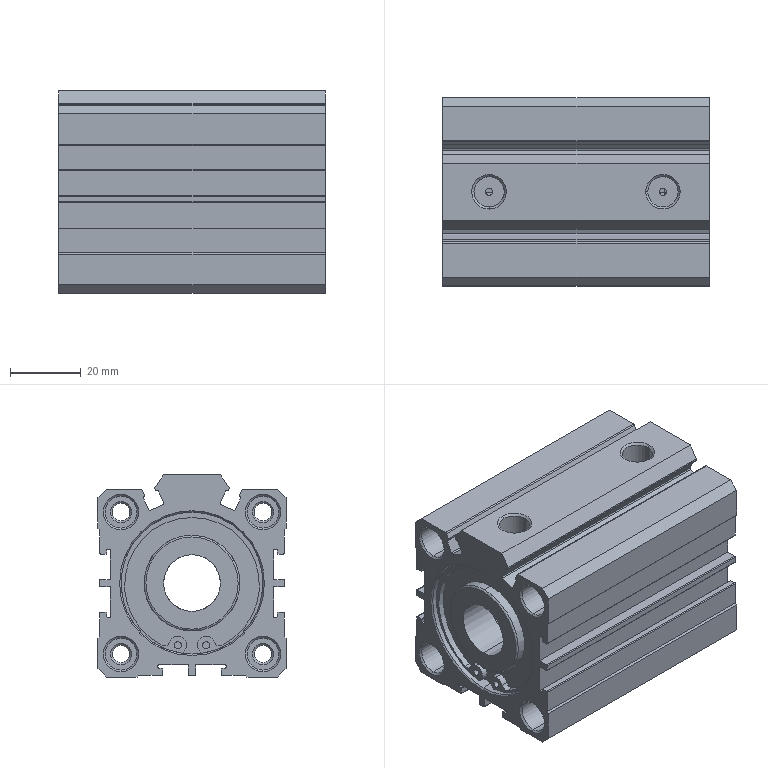Part | STEP file | ASND-0110-ACQDS-40x25-G-21aq | 1 solid | 255 faces | box 75 x 53 x 57 mm | volume 115109 mm3 | cylinder 117 | plane 94 | cone 40 | torus 4 | commonest cylinder face diameters 0.4 x36 9 x16 0.8 x12 2 x12 4.917 x8 3 x6